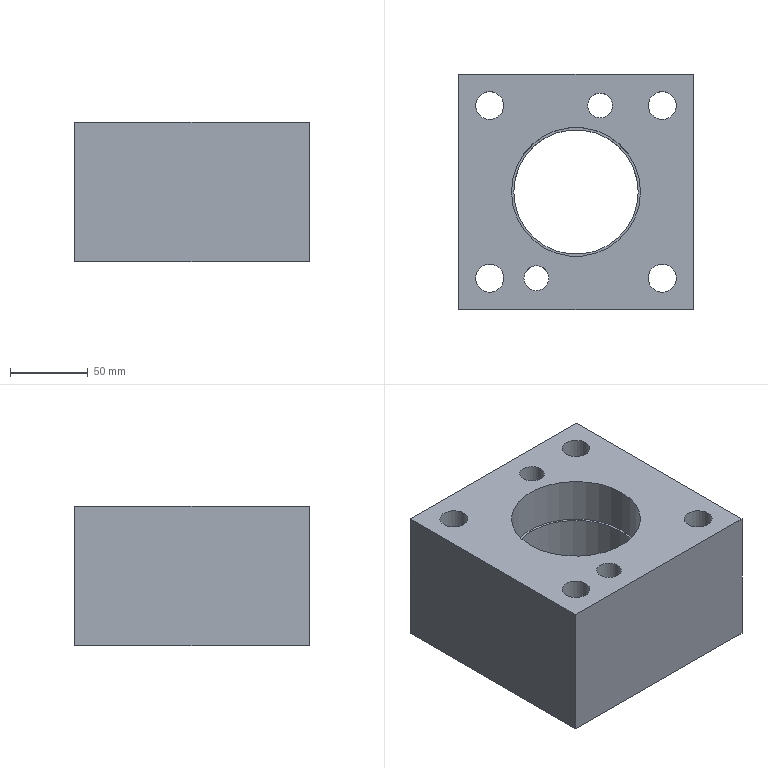Part | STEP file | lll_id766_x_t | 1 solid | 39 faces | box 151 x 151 x 90 mm | volume 1390274 mm3 | cylinder 20 | plane 13 | cone 6 | commonest cylinder face diameters 6.806 x4 18.009 x4 26.007 x4 10.505 x2 16 x2 18.5 x2
STEP:
#1=CARTESIAN_POINT('',(398.807,491.144,72.5));
#2=VERTEX_POINT('',#1);
#3=CARTESIAN_POINT('',(402.21,491.144,72.5));
#4=DIRECTION('',(0.,0.,-1.));
#5=DIRECTION('',(-1.,0.,0.));
#6=AXIS2_PLACEMENT_3D('',#3,#4,#5);
#7=CIRCLE('',#6,3.403);
#8=EDGE_CURVE('',#2,#2,#7,.T.);
#9=ORIENTED_EDGE('',*,*,#8,.F.);
#10=EDGE_LOOP('',(#9));
#11=FACE_BOUND('',#10,.T.);
#12=CARTESIAN_POINT('',(440.176,550.225,72.5));
#13=VERTEX_POINT('',#12);
#14=CARTESIAN_POINT('',(443.579,550.225,72.5));
#15=DIRECTION('',(0.,0.,-1.));
#16=DIRECTION('',(-1.,0.,0.));
#17=AXIS2_PLACEMENT_3D('',#14,#15,#16);
#18=CIRCLE('',#17,3.403);
#19=EDGE_CURVE('',#13,#13,#18,.T.);
#20=ORIENTED_EDGE('',*,*,#19,.F.);
#21=EDGE_LOOP('',(#20));
#22=FACE_BOUND('',#21,.T.);
#23=CARTESIAN_POINT('',(499.257,508.856,72.5));
#24=VERTEX_POINT('',#23);
#25=CARTESIAN_POINT('',(502.66,508.856,72.5));
#26=DIRECTION('',(0.,0.,-1.));
#27=DIRECTION('',(-1.,0.,0.));
#28=AXIS2_PLACEMENT_3D('',#25,#26,#27);
#29=CIRCLE('',#28,3.403);
#30=EDGE_CURVE('',#24,#24,#29,.T.);
#31=ORIENTED_EDGE('',*,*,#30,.F.);
#32=EDGE_LOOP('',(#31));
#33=FACE_BOUND('',#32,.T.);
#34=CARTESIAN_POINT('',(457.888,449.775,72.5));
#35=VERTEX_POINT('',#34);
#36=CARTESIAN_POINT('',(461.291,449.775,72.5));
#37=DIRECTION('',(0.,0.,-1.));
#38=DIRECTION('',(-1.,0.,0.));
#39=AXIS2_PLACEMENT_3D('',#36,#37,#38);
#40=CIRCLE('',#39,3.403);
#41=EDGE_CURVE('',#35,#35,#40,.T.);
#42=ORIENTED_EDGE('',*,*,#41,.F.);
#43=EDGE_LOOP('',(#42));
#44=FACE_BOUND('',#43,.T.);
#45=CARTESIAN_POINT('',(417.685,444.5,72.5));
#46=VERTEX_POINT('',#45);
#47=CARTESIAN_POINT('',(426.935,444.5,72.5));
#48=DIRECTION('',(0.,0.,-1.));
#49=DIRECTION('',(-1.,0.,0.));
#50=AXIS2_PLACEMENT_3D('',#47,#48,#49);
#51=CIRCLE('',#50,9.25);
#52=EDGE_CURVE('',#46,#46,#51,.T.);
#53=ORIENTED_EDGE('',*,*,#52,.F.);
#54=EDGE_LOOP('',(#53));
#55=FACE_BOUND('',#54,.T.);
#56=CARTESIAN_POINT('',(409.939,555.5,72.5));
#57=VERTEX_POINT('',#56);
#58=CARTESIAN_POINT('',(396.935,555.5,72.5));
#59=DIRECTION('',(0.,0.,1.));
#60=DIRECTION('',(1.,0.,0.));
#61=AXIS2_PLACEMENT_3D('',#58,#59,#60);
#62=CIRCLE('',#61,13.004);
#63=EDGE_CURVE('',#57,#57,#62,.T.);
#64=ORIENTED_EDGE('',*,*,#63,.T.);
#65=EDGE_LOOP('',(#64));
#66=FACE_BOUND('',#65,.T.);
#67=CARTESIAN_POINT('',(458.685,555.5,72.5));
#68=VERTEX_POINT('',#67);
#69=CARTESIAN_POINT('',(467.935,555.5,72.5));
#70=DIRECTION('',(0.,0.,-1.));
#71=DIRECTION('',(-1.,0.,0.));
#72=AXIS2_PLACEMENT_3D('',#69,#70,#71);
#73=CIRCLE('',#72,9.25);
#74=EDGE_CURVE('',#68,#68,#73,.T.);
#75=ORIENTED_EDGE('',*,*,#74,.F.);
#76=EDGE_LOOP('',(#75));
#77=FACE_BOUND('',#76,.T.);
#78=CARTESIAN_POINT('',(520.939,444.5,72.5));
#79=VERTEX_POINT('',#78);
#80=CARTESIAN_POINT('',(507.935,444.5,72.5));
#81=DIRECTION('',(0.,0.,1.));
#82=DIRECTION('',(1.,0.,0.));
#83=AXIS2_PLACEMENT_3D('',#80,#81,#82);
#84=CIRCLE('',#83,13.004);
#85=EDGE_CURVE('',#79,#79,#84,.T.);
#86=ORIENTED_EDGE('',*,*,#85,.T.);
#87=EDGE_LOOP('',(#86));
#88=FACE_BOUND('',#87,.T.);
#89=CARTESIAN_POINT('',(417.683,559.5,72.5));
#90=VERTEX_POINT('',#89);
#91=CARTESIAN_POINT('',(422.935,559.5,72.5));
#92=DIRECTION('',(0.,0.,-1.));
#93=DIRECTION('',(-1.,0.,0.));
#94=AXIS2_PLACEMENT_3D('',#91,#92,#93);
#95=CIRCLE('',#94,5.253);
#96=EDGE_CURVE('',#90,#90,#95,.T.);
#97=ORIENTED_EDGE('',*,*,#96,.F.);
#98=EDGE_LOOP('',(#97));
#99=FACE_BOUND('',#98,.T.);
#100=CARTESIAN_POINT('',(476.683,440.5,72.5));
#101=VERTEX_POINT('',#100);
#102=CARTESIAN_POINT('',(481.935,440.5,72.5));
#103=DIRECTION('',(0.,0.,-1.));
#104=DIRECTION('',(-1.,0.,0.));
#105=AXIS2_PLACEMENT_3D('',#102,#103,#104);
#106=CIRCLE('',#105,5.253);
#107=EDGE_CURVE('',#101,#101,#106,.T.);
#108=ORIENTED_EDGE('',*,*,#107,.F.);
#109=EDGE_LOOP('',(#108));
#110=FACE_BOUND('',#109,.T.);
#111=CARTESIAN_POINT('',(376.935,424.5,72.5));
#112=VERTEX_POINT('',#111);
#113=CARTESIAN_POINT('',(527.935,424.5,72.5));
#114=VERTEX_POINT('',#113);
#115=CARTESIAN_POINT('',(452.435,424.5,72.5));
#116=DIRECTION('',(1.,0.,0.));
#117=VECTOR('',#116,1.);
#118=LINE('',#115,#117);
#119=EDGE_CURVE('',#112,#114,#118,.T.);
#120=ORIENTED_EDGE('',*,*,#119,.F.);
#121=CARTESIAN_POINT('',(376.935,575.5,72.5));
#122=VERTEX_POINT('',#121);
#123=CARTESIAN_POINT('',(376.935,0.,72.5));
#124=DIRECTION('',(0.,1.,0.));
#125=VECTOR('',#124,1.);
#126=LINE('',#123,#125);
#127=EDGE_CURVE('',#112,#122,#126,.T.);
#128=ORIENTED_EDGE('',*,*,#127,.T.);
#129=CARTESIAN_POINT('',(527.935,575.5,72.5));
#130=VERTEX_POINT('',#129);
#131=CARTESIAN_POINT('',(452.435,575.5,72.5));
#132=DIRECTION('',(-1.,0.,0.));
#133=VECTOR('',#132,1.);
#134=LINE('',#131,#133);
#135=EDGE_CURVE('',#130,#122,#134,.T.);
#136=ORIENTED_EDGE('',*,*,#135,.F.);
#137=CARTESIAN_POINT('',(527.935,0.,72.5));
#138=DIRECTION('',(0.,-1.,0.));
#139=VECTOR('',#138,1.);
#140=LINE('',#137,#139);
#141=EDGE_CURVE('',#130,#114,#140,.T.);
#142=ORIENTED_EDGE('',*,*,#141,.T.);
#143=EDGE_LOOP('',(#120,#128,#136,#142));
#144=FACE_BOUND('',#143,.T.);
#145=CARTESIAN_POINT('',(492.435,500.,72.5));
#146=VERTEX_POINT('',#145);
#147=CARTESIAN_POINT('',(452.435,500.,72.5));
#148=DIRECTION('',(0.,0.,1.));
#149=DIRECTION('',(1.,0.,0.));
#150=AXIS2_PLACEMENT_3D('',#147,#148,#149);
#151=CIRCLE('',#150,40.);
#152=EDGE_CURVE('',#146,#146,#151,.T.);
#153=ORIENTED_EDGE('',*,*,#152,.T.);
#154=EDGE_LOOP('',(#153));
#155=FACE_BOUND('',#154,.T.);
#156=CARTESIAN_POINT('',(520.939,555.5,72.5));
#157=VERTEX_POINT('',#156);
#158=CARTESIAN_POINT('',(507.935,555.5,72.5));
#159=DIRECTION('',(0.,0.,1.));
#160=DIRECTION('',(1.,0.,0.));
#161=AXIS2_PLACEMENT_3D('',#158,#159,#160);
#162=CIRCLE('',#161,13.004);
#163=EDGE_CURVE('',#157,#157,#162,.T.);
#164=ORIENTED_EDGE('',*,*,#163,.T.);
#165=EDGE_LOOP('',(#164));
#166=FACE_BOUND('',#165,.T.);
#167=CARTESIAN_POINT('',(409.939,444.5,72.5));
#168=VERTEX_POINT('',#167);
#169=CARTESIAN_POINT('',(396.935,444.5,72.5));
#170=DIRECTION('',(0.,0.,1.));
#171=DIRECTION('',(1.,0.,0.));
#172=AXIS2_PLACEMENT_3D('',#169,#170,#171);
#173=CIRCLE('',#172,13.004);
#174=EDGE_CURVE('',#168,#168,#173,.T.);
#175=ORIENTED_EDGE('',*,*,#174,.T.);
#176=EDGE_LOOP('',(#175));
#177=FACE_BOUND('',#176,.T.);
#178=CARTESIAN_POINT('',(2067.435,0.,72.5));
#179=DIRECTION('',(0.,0.,-1.));
#180=DIRECTION('',(-1.,0.,0.));
#181=AXIS2_PLACEMENT_3D('',#178,#179,#180);
#182=PLANE('',#181);
#183=ADVANCED_FACE('',(#11,#22,#33,#44,#55,#66,#77,#88,#99,#110,#144,#155,#166,#177),#182,.T.);
#184=CARTESIAN_POINT('',(418.935,444.5,162.5));
#185=VERTEX_POINT('',#184);
#186=CARTESIAN_POINT('',(426.935,444.5,162.5));
#187=DIRECTION('',(0.,0.,-1.));
#188=DIRECTION('',(-1.,0.,0.));
#189=AXIS2_PLACEMENT_3D('',#186,#187,#188);
#190=CIRCLE('',#189,8.);
#191=EDGE_CURVE('',#185,#185,#190,.T.);
#192=ORIENTED_EDGE('',*,*,#191,.T.);
#193=EDGE_LOOP('',(#192));
#194=FACE_BOUND('',#193,.T.);
#195=CARTESIAN_POINT('',(387.931,444.5,162.5));
#196=VERTEX_POINT('',#195);
#197=CARTESIAN_POINT('',(396.935,444.5,162.5));
#198=DIRECTION('',(0.,0.,-1.));
#199=DIRECTION('',(-1.,0.,0.));
#200=AXIS2_PLACEMENT_3D('',#197,#198,#199);
#201=CIRCLE('',#200,9.005);
#202=EDGE_CURVE('',#196,#196,#201,.T.);
#203=ORIENTED_EDGE('',*,*,#202,.T.);
#204=EDGE_LOOP('',(#203));
#205=FACE_BOUND('',#204,.T.);
#206=CARTESIAN_POINT('',(387.931,555.5,162.5));
#207=VERTEX_POINT('',#206);
#208=CARTESIAN_POINT('',(396.935,555.5,162.5));
#209=DIRECTION('',(0.,0.,-1.));
#210=DIRECTION('',(-1.,0.,0.));
#211=AXIS2_PLACEMENT_3D('',#208,#209,#210);
#212=CIRCLE('',#211,9.005);
#213=EDGE_CURVE('',#207,#207,#212,.T.);
#214=ORIENTED_EDGE('',*,*,#213,.T.);
#215=EDGE_LOOP('',(#214));
#216=FACE_BOUND('',#215,.T.);
#217=CARTESIAN_POINT('',(459.935,555.5,162.5));
#218=VERTEX_POINT('',#217);
#219=CARTESIAN_POINT('',(467.935,555.5,162.5));
#220=DIRECTION('',(0.,0.,-1.));
#221=DIRECTION('',(-1.,0.,0.));
#222=AXIS2_PLACEMENT_3D('',#219,#220,#221);
#223=CIRCLE('',#222,8.);
#224=EDGE_CURVE('',#218,#218,#223,.T.);
#225=ORIENTED_EDGE('',*,*,#224,.T.);
#226=EDGE_LOOP('',(#225));
#227=FACE_BOUND('',#226,.T.);
#228=CARTESIAN_POINT('',(498.931,555.5,162.5));
#229=VERTEX_POINT('',#228);
#230=CARTESIAN_POINT('',(507.935,555.5,162.5));
#231=DIRECTION('',(0.,0.,-1.));
#232=DIRECTION('',(-1.,0.,0.));
#233=AXIS2_PLACEMENT_3D('',#230,#231,#232);
#234=CIRCLE('',#233,9.005);
#235=EDGE_CURVE('',#229,#229,#234,.T.);
#236=ORIENTED_EDGE('',*,*,#235,.T.);
#237=EDGE_LOOP('',(#236));
#238=FACE_BOUND('',#237,.T.);
#239=CARTESIAN_POINT('',(498.931,444.5,162.5));
#240=VERTEX_POINT('',#239);
#241=CARTESIAN_POINT('',(507.935,444.5,162.5));
#242=DIRECTION('',(0.,0.,-1.));
#243=DIRECTION('',(-1.,0.,0.));
#244=AXIS2_PLACEMENT_3D('',#241,#242,#243);
#245=CIRCLE('',#244,9.005);
#246=EDGE_CURVE('',#240,#240,#245,.T.);
#247=ORIENTED_EDGE('',*,*,#246,.T.);
#248=EDGE_LOOP('',(#247));
#249=FACE_BOUND('',#248,.T.);
#250=CARTESIAN_POINT('',(410.935,500.,162.5));
#251=VERTEX_POINT('',#250);
#252=CARTESIAN_POINT('',(452.435,500.,162.5));
#253=DIRECTION('',(0.,0.,-1.));
#254=DIRECTION('',(-1.,0.,0.));
#255=AXIS2_PLACEMENT_3D('',#252,#253,#254);
#256=CIRCLE('',#255,41.5);
#257=EDGE_CURVE('',#251,#251,#256,.T.);
#258=ORIENTED_EDGE('',*,*,#257,.T.);
#259=EDGE_LOOP('',(#258));
#260=FACE_BOUND('',#259,.T.);
#261=CARTESIAN_POINT('',(527.935,424.5,162.5));
#262=VERTEX_POINT('',#261);
#263=CARTESIAN_POINT('',(376.935,424.5,162.5));
#264=VERTEX_POINT('',#263);
#265=CARTESIAN_POINT('',(2067.435,424.5,162.5));
#266=DIRECTION('',(-1.,0.,0.));
#267=VECTOR('',#266,1.);
#268=LINE('',#265,#267);
#269=EDGE_CURVE('',#262,#264,#268,.T.);
#270=ORIENTED_EDGE('',*,*,#269,.F.);
#271=CARTESIAN_POINT('',(527.935,575.5,162.5));
#272=VERTEX_POINT('',#271);
#273=CARTESIAN_POINT('',(527.935,500.,162.5));
#274=DIRECTION('',(0.,1.,0.));
#275=VECTOR('',#274,1.);
#276=LINE('',#273,#275);
#277=EDGE_CURVE('',#262,#272,#276,.T.);
#278=ORIENTED_EDGE('',*,*,#277,.T.);
#279=CARTESIAN_POINT('',(376.935,575.5,162.5));
#280=VERTEX_POINT('',#279);
#281=CARTESIAN_POINT('',(452.435,575.5,162.5));
#282=DIRECTION('',(-1.,0.,0.));
#283=VECTOR('',#282,1.);
#284=LINE('',#281,#283);
#285=EDGE_CURVE('',#272,#280,#284,.T.);
#286=ORIENTED_EDGE('',*,*,#285,.T.);
#287=CARTESIAN_POINT('',(376.935,500.,162.5));
#288=DIRECTION('',(0.,-1.,0.));
#289=VECTOR('',#288,1.);
#290=LINE('',#287,#289);
#291=EDGE_CURVE('',#280,#264,#290,.T.);
#292=ORIENTED_EDGE('',*,*,#291,.T.);
#293=EDGE_LOOP('',(#270,#278,#286,#292));
#294=FACE_BOUND('',#293,.T.);
#295=CARTESIAN_POINT('',(2067.435,0.,162.5));
#296=DIRECTION('',(0.,0.,-1.));
#297=DIRECTION('',(-1.,0.,0.));
#298=AXIS2_PLACEMENT_3D('',#295,#296,#297);
#299=PLANE('',#298);
#300=ADVANCED_FACE('',(#194,#205,#216,#227,#238,#249,#260,#294),#299,.F.);
#301=CARTESIAN_POINT('',(527.935,424.5,89.));
#302=DIRECTION('',(0.,0.,1.));
#303=VECTOR('',#302,1.);
#304=LINE('',#301,#303);
#305=EDGE_CURVE('',#114,#262,#304,.T.);
#306=ORIENTED_EDGE('',*,*,#305,.F.);
#307=ORIENTED_EDGE('',*,*,#141,.F.);
#308=CARTESIAN_POINT('',(527.935,575.5,89.));
#309=DIRECTION('',(0.,0.,1.));
#310=VECTOR('',#309,1.);
#311=LINE('',#308,#310);
#312=EDGE_CURVE('',#130,#272,#311,.T.);
#313=ORIENTED_EDGE('',*,*,#312,.T.);
#314=ORIENTED_EDGE('',*,*,#277,.F.);
#315=EDGE_LOOP('',(#306,#307,#313,#314));
#316=FACE_OUTER_BOUND('',#315,.T.);
#317=CARTESIAN_POINT('',(527.935,500.,89.));
#318=DIRECTION('',(1.,0.,0.));
#319=DIRECTION('',(0.,0.,-1.));
#320=AXIS2_PLACEMENT_3D('',#317,#318,#319);
#321=PLANE('',#320);
#322=ADVANCED_FACE('',(#316),#321,.T.);
#323=ORIENTED_EDGE('',*,*,#312,.F.);
#324=ORIENTED_EDGE('',*,*,#135,.T.);
#325=CARTESIAN_POINT('',(376.935,575.5,89.));
#326=DIRECTION('',(0.,0.,1.));
#327=VECTOR('',#326,1.);
#328=LINE('',#325,#327);
#329=EDGE_CURVE('',#122,#280,#328,.T.);
#330=ORIENTED_EDGE('',*,*,#329,.T.);
#331=ORIENTED_EDGE('',*,*,#285,.F.);
#332=EDGE_LOOP('',(#323,#324,#330,#331));
#333=FACE_OUTER_BOUND('',#332,.T.);
#334=CARTESIAN_POINT('',(452.435,575.5,89.));
#335=DIRECTION('',(0.,1.,0.));
#336=DIRECTION('',(0.,0.,1.));
#337=AXIS2_PLACEMENT_3D('',#334,#335,#336);
#338=PLANE('',#337);
#339=ADVANCED_FACE('',(#333),#338,.T.);
#340=ORIENTED_EDGE('',*,*,#329,.F.);
#341=ORIENTED_EDGE('',*,*,#127,.F.);
#342=CARTESIAN_POINT('',(376.935,424.5,89.));
#343=DIRECTION('',(0.,0.,1.));
#344=VECTOR('',#343,1.);
#345=LINE('',#342,#344);
#346=EDGE_CURVE('',#112,#264,#345,.T.);
#347=ORIENTED_EDGE('',*,*,#346,.T.);
#348=ORIENTED_EDGE('',*,*,#291,.F.);
#349=EDGE_LOOP('',(#340,#341,#347,#348));
#350=FACE_OUTER_BOUND('',#349,.T.);
#351=CARTESIAN_POINT('',(376.935,500.,89.));
#352=DIRECTION('',(-1.,0.,0.));
#353=DIRECTION('',(0.,0.,1.));
#354=AXIS2_PLACEMENT_3D('',#351,#352,#353);
#355=PLANE('',#354);
#356=ADVANCED_FACE('',(#350),#355,.T.);
#357=ORIENTED_EDGE('',*,*,#346,.F.);
#358=ORIENTED_EDGE('',*,*,#119,.T.);
#359=ORIENTED_EDGE('',*,*,#305,.T.);
#360=ORIENTED_EDGE('',*,*,#269,.T.);
#361=EDGE_LOOP('',(#357,#358,#359,#360));
#362=FACE_OUTER_BOUND('',#361,.T.);
#363=CARTESIAN_POINT('',(452.435,424.5,89.));
#364=DIRECTION('',(0.,-1.,0.));
#365=DIRECTION('',(0.,0.,-1.));
#366=AXIS2_PLACEMENT_3D('',#363,#364,#365);
#367=PLANE('',#366);
#368=ADVANCED_FACE('',(#362),#367,.T.);
#369=CARTESIAN_POINT('',(492.435,500.,133.));
#370=VERTEX_POINT('',#369);
#371=CARTESIAN_POINT('',(452.435,500.,133.));
#372=DIRECTION('',(0.,0.,-1.));
#373=DIRECTION('',(1.,0.,0.));
#374=AXIS2_PLACEMENT_3D('',#371,#372,#373);
#375=CIRCLE('',#374,40.);
#376=EDGE_CURVE('',#370,#370,#375,.T.);
#377=ORIENTED_EDGE('',*,*,#376,.F.);
#378=EDGE_LOOP('',(#377));
#379=FACE_BOUND('',#378,.T.);
#380=ORIENTED_EDGE('',*,*,#152,.F.);
#381=EDGE_LOOP('',(#380));
#382=FACE_BOUND('',#381,.T.);
#383=CARTESIAN_POINT('',(452.435,500.,317.5));
#384=DIRECTION('',(0.,0.,-1.));
#385=DIRECTION('',(-1.,0.,0.));
#386=AXIS2_PLACEMENT_3D('',#383,#384,#385);
#387=CYLINDRICAL_SURFACE('',#386,40.);
#388=ADVANCED_FACE('',(#379,#382),#387,.F.);
#389=CARTESIAN_POINT('',(493.935,500.,133.));
#390=VERTEX_POINT('',#389);
#391=CARTESIAN_POINT('',(452.435,500.,133.));
#392=DIRECTION('',(0.,0.,-1.));
#393=DIRECTION('',(1.,0.,0.));
#394=AXIS2_PLACEMENT_3D('',#391,#392,#393);
#395=CIRCLE('',#394,41.5);
#396=EDGE_CURVE('',#390,#390,#395,.T.);
#397=ORIENTED_EDGE('',*,*,#396,.T.);
#398=EDGE_LOOP('',(#397));
#399=FACE_BOUND('',#398,.T.);
#400=ORIENTED_EDGE('',*,*,#257,.F.);
#401=EDGE_LOOP('',(#400));
#402=FACE_BOUND('',#401,.T.);
#403=CARTESIAN_POINT('',(452.435,500.,153.));
#404=DIRECTION('',(0.,0.,-1.));
#405=DIRECTION('',(-1.,0.,0.));
#406=AXIS2_PLACEMENT_3D('',#403,#404,#405);
#407=CYLINDRICAL_SURFACE('',#406,41.5);
#408=ADVANCED_FACE('',(#399,#402),#407,.F.);
#409=ORIENTED_EDGE('',*,*,#376,.T.);
#410=EDGE_LOOP('',(#409));
#411=FACE_BOUND('',#410,.T.);
#412=ORIENTED_EDGE('',*,*,#396,.F.);
#413=EDGE_LOOP('',(#412));
#414=FACE_BOUND('',#413,.T.);
#415=CARTESIAN_POINT('',(452.435,500.,133.));
#416=DIRECTION('',(0.,0.,1.));
#417=DIRECTION('',(-1.,0.,0.));
#418=AXIS2_PLACEMENT_3D('',#415,#416,#417);
#419=PLANE('',#418);
#420=ADVANCED_FACE('',(#411,#414),#419,.T.);
#421=ORIENTED_EDGE('',*,*,#107,.T.);
#422=EDGE_LOOP('',(#421));
#423=FACE_BOUND('',#422,.T.);
#424=CARTESIAN_POINT('',(487.188,440.5,102.253));
#425=VERTEX_POINT('',#424);
#426=CARTESIAN_POINT('',(481.935,440.5,102.253));
#427=DIRECTION('',(0.,0.,1.));
#428=DIRECTION('',(1.,0.,0.));
#429=AXIS2_PLACEMENT_3D('',#426,#427,#428);
#430=CIRCLE('',#429,5.253);
#431=EDGE_CURVE('',#425,#425,#430,.T.);
#432=ORIENTED_EDGE('',*,*,#431,.T.);
#433=EDGE_LOOP('',(#432));
#434=FACE_BOUND('',#433,.T.);
#435=CARTESIAN_POINT('',(481.935,440.5,67.5));
#436=DIRECTION('',(0.,0.,1.));
#437=DIRECTION('',(1.,0.,0.));
#438=AXIS2_PLACEMENT_3D('',#435,#436,#437);
#439=CYLINDRICAL_SURFACE('',#438,5.253);
#440=ADVANCED_FACE('',(#423,#434),#439,.F.);
#441=CARTESIAN_POINT('',(481.935,440.5,107.506));
#442=VERTEX_POINT('',#441);
#443=VERTEX_LOOP('',#442);
#444=FACE_BOUND('',#443,.T.);
#445=ORIENTED_EDGE('',*,*,#431,.F.);
#446=EDGE_LOOP('',(#445));
#447=FACE_BOUND('',#446,.T.);
#448=CARTESIAN_POINT('',(481.935,440.5,102.253));
#449=DIRECTION('',(0.,0.,-1.));
#450=DIRECTION('',(-1.,0.,0.));
#451=AXIS2_PLACEMENT_3D('',#448,#449,#450);
#452=CONICAL_SURFACE('',#451,5.253,45.);
#453=ADVANCED_FACE('',(#444,#447),#452,.F.);
#454=ORIENTED_EDGE('',*,*,#96,.T.);
#455=EDGE_LOOP('',(#454));
#456=FACE_BOUND('',#455,.T.);
#457=CARTESIAN_POINT('',(428.188,559.5,102.253));
#458=VERTEX_POINT('',#457);
#459=CARTESIAN_POINT('',(422.935,559.5,102.253));
#460=DIRECTION('',(0.,0.,1.));
#461=DIRECTION('',(1.,0.,0.));
#462=AXIS2_PLACEMENT_3D('',#459,#460,#461);
#463=CIRCLE('',#462,5.253);
#464=EDGE_CURVE('',#458,#458,#463,.T.);
#465=ORIENTED_EDGE('',*,*,#464,.T.);
#466=EDGE_LOOP('',(#465));
#467=FACE_BOUND('',#466,.T.);
#468=CARTESIAN_POINT('',(422.935,559.5,67.5));
#469=DIRECTION('',(0.,0.,1.));
#470=DIRECTION('',(1.,0.,0.));
#471=AXIS2_PLACEMENT_3D('',#468,#469,#470);
#472=CYLINDRICAL_SURFACE('',#471,5.253);
#473=ADVANCED_FACE('',(#456,#467),#472,.F.);
#474=CARTESIAN_POINT('',(422.935,559.5,107.506));
#475=VERTEX_POINT('',#474);
#476=VERTEX_LOOP('',#475);
#477=FACE_BOUND('',#476,.T.);
#478=ORIENTED_EDGE('',*,*,#464,.F.);
#479=EDGE_LOOP('',(#478));
#480=FACE_BOUND('',#479,.T.);
#481=CARTESIAN_POINT('',(422.935,559.5,102.253));
#482=DIRECTION('',(0.,0.,-1.));
#483=DIRECTION('',(-1.,0.,0.));
#484=AXIS2_PLACEMENT_3D('',#481,#482,#483);
#485=CONICAL_SURFACE('',#484,5.253,45.);
#486=ADVANCED_FACE('',(#477,#480),#485,.F.);
#487=CARTESIAN_POINT('',(516.94,444.5,122.5));
#488=VERTEX_POINT('',#487);
#489=CARTESIAN_POINT('',(507.935,444.5,122.5));
#490=DIRECTION('',(0.,0.,1.));
#491=DIRECTION('',(1.,0.,0.));
#492=AXIS2_PLACEMENT_3D('',#489,#490,#491);
#493=CIRCLE('',#492,9.005);
#494=EDGE_CURVE('',#488,#488,#493,.T.);
#495=ORIENTED_EDGE('',*,*,#494,.F.);
#496=EDGE_LOOP('',(#495));
#497=FACE_BOUND('',#496,.T.);
#498=ORIENTED_EDGE('',*,*,#246,.F.);
#499=EDGE_LOOP('',(#498));
#500=FACE_BOUND('',#499,.T.);
#501=CARTESIAN_POINT('',(507.935,444.5,67.5));
#502=DIRECTION('',(0.,0.,1.));
#503=DIRECTION('',(-1.,0.,0.));
#504=AXIS2_PLACEMENT_3D('',#501,#502,#503);
#505=CYLINDRICAL_SURFACE('',#504,9.005);
#506=ADVANCED_FACE('',(#497,#500),#505,.F.);
#507=ORIENTED_EDGE('',*,*,#494,.T.);
#508=EDGE_LOOP('',(#507));
#509=FACE_BOUND('',#508,.T.);
#510=CARTESIAN_POINT('',(520.939,444.5,122.5));
#511=VERTEX_POINT('',#510);
#512=CARTESIAN_POINT('',(507.935,444.5,122.5));
#513=DIRECTION('',(0.,0.,1.));
#514=DIRECTION('',(1.,0.,0.));
#515=AXIS2_PLACEMENT_3D('',#512,#513,#514);
#516=CIRCLE('',#515,13.004);
#517=EDGE_CURVE('',#511,#511,#516,.T.);
#518=ORIENTED_EDGE('',*,*,#517,.F.);
#519=EDGE_LOOP('',(#518));
#520=FACE_BOUND('',#519,.T.);
#521=CARTESIAN_POINT('',(507.935,444.5,122.5));
#522=DIRECTION('',(0.,0.,1.));
#523=DIRECTION('',(-1.,0.,0.));
#524=AXIS2_PLACEMENT_3D('',#521,#522,#523);
#525=PLANE('',#524);
#526=ADVANCED_FACE('',(#509,#520),#525,.F.);
#527=ORIENTED_EDGE('',*,*,#517,.T.);
#528=EDGE_LOOP('',(#527));
#529=FACE_BOUND('',#528,.T.);
#530=ORIENTED_EDGE('',*,*,#85,.F.);
#531=EDGE_LOOP('',(#530));
#532=FACE_BOUND('',#531,.T.);
#533=CARTESIAN_POINT('',(507.935,444.5,72.5));
#534=DIRECTION('',(0.,0.,1.));
#535=DIRECTION('',(-1.,0.,0.));
#536=AXIS2_PLACEMENT_3D('',#533,#534,#535);
#537=CYLINDRICAL_SURFACE('',#536,13.004);
#538=ADVANCED_FACE('',(#529,#532),#537,.F.);
#539=CARTESIAN_POINT('',(516.94,555.5,122.5));
#540=VERTEX_POINT('',#539);
#541=CARTESIAN_POINT('',(507.935,555.5,122.5));
#542=DIRECTION('',(0.,0.,1.));
#543=DIRECTION('',(1.,0.,0.));
#544=AXIS2_PLACEMENT_3D('',#541,#542,#543);
#545=CIRCLE('',#544,9.005);
#546=EDGE_CURVE('',#540,#540,#545,.T.);
#547=ORIENTED_EDGE('',*,*,#546,.F.);
#548=EDGE_LOOP('',(#547));
#549=FACE_BOUND('',#548,.T.);
#550=ORIENTED_EDGE('',*,*,#235,.F.);
#551=EDGE_LOOP('',(#550));
#552=FACE_BOUND('',#551,.T.);
#553=CARTESIAN_POINT('',(507.935,555.5,67.5));
#554=DIRECTION('',(0.,0.,1.));
#555=DIRECTION('',(-1.,0.,0.));
#556=AXIS2_PLACEMENT_3D('',#553,#554,#555);
#557=CYLINDRICAL_SURFACE('',#556,9.005);
#558=ADVANCED_FACE('',(#549,#552),#557,.F.);
#559=ORIENTED_EDGE('',*,*,#546,.T.);
#560=EDGE_LOOP('',(#559));
#561=FACE_BOUND('',#560,.T.);
#562=CARTESIAN_POINT('',(520.939,555.5,122.5));
#563=VERTEX_POINT('',#562);
#564=CARTESIAN_POINT('',(507.935,555.5,122.5));
#565=DIRECTION('',(0.,0.,1.));
#566=DIRECTION('',(1.,0.,0.));
#567=AXIS2_PLACEMENT_3D('',#564,#565,#566);
#568=CIRCLE('',#567,13.004);
#569=EDGE_CURVE('',#563,#563,#568,.T.);
#570=ORIENTED_EDGE('',*,*,#569,.F.);
#571=EDGE_LOOP('',(#570));
#572=FACE_BOUND('',#571,.T.);
#573=CARTESIAN_POINT('',(507.935,555.5,122.5));
#574=DIRECTION('',(0.,0.,1.));
#575=DIRECTION('',(-1.,0.,0.));
#576=AXIS2_PLACEMENT_3D('',#573,#574,#575);
#577=PLANE('',#576);
#578=ADVANCED_FACE('',(#561,#572),#577,.F.);
#579=ORIENTED_EDGE('',*,*,#569,.T.);
#580=EDGE_LOOP('',(#579));
#581=FACE_BOUND('',#580,.T.);
#582=ORIENTED_EDGE('',*,*,#163,.F.);
#583=EDGE_LOOP('',(#582));
#584=FACE_BOUND('',#583,.T.);
#585=CARTESIAN_POINT('',(507.935,555.5,72.5));
#586=DIRECTION('',(0.,0.,1.));
#587=DIRECTION('',(-1.,0.,0.));
#588=AXIS2_PLACEMENT_3D('',#585,#586,#587);
#589=CYLINDRICAL_SURFACE('',#588,13.004);
#590=ADVANCED_FACE('',(#581,#584),#589,.F.);
#591=CARTESIAN_POINT('',(475.935,555.5,113.5));
#592=VERTEX_POINT('',#591);
#593=CARTESIAN_POINT('',(467.935,555.5,113.5));
#594=DIRECTION('',(0.,0.,1.));
#595=DIRECTION('',(1.,0.,0.));
#596=AXIS2_PLACEMENT_3D('',#593,#594,#595);
#597=CIRCLE('',#596,8.);
#598=EDGE_CURVE('',#592,#592,#597,.T.);
#599=ORIENTED_EDGE('',*,*,#598,.F.);
#600=EDGE_LOOP('',(#599));
#601=FACE_BOUND('',#600,.T.);
#602=ORIENTED_EDGE('',*,*,#224,.F.);
#603=EDGE_LOOP('',(#602));
#604=FACE_BOUND('',#603,.T.);
#605=CARTESIAN_POINT('',(467.935,555.5,67.5));
#606=DIRECTION('',(0.,0.,1.));
#607=DIRECTION('',(-1.,0.,0.));
#608=AXIS2_PLACEMENT_3D('',#605,#606,#607);
#609=CYLINDRICAL_SURFACE('',#608,8.);
#610=ADVANCED_FACE('',(#601,#604),#609,.F.);
#611=ORIENTED_EDGE('',*,*,#598,.T.);
#612=EDGE_LOOP('',(#611));
#613=FACE_BOUND('',#612,.T.);
#614=CARTESIAN_POINT('',(477.185,555.5,113.5));
#615=VERTEX_POINT('',#614);
#616=CARTESIAN_POINT('',(467.935,555.5,113.5));
#617=DIRECTION('',(0.,0.,1.));
#618=DIRECTION('',(1.,0.,0.));
#619=AXIS2_PLACEMENT_3D('',#616,#617,#618);
#620=CIRCLE('',#619,9.25);
#621=EDGE_CURVE('',#615,#615,#620,.T.);
#622=ORIENTED_EDGE('',*,*,#621,.F.);
#623=EDGE_LOOP('',(#622));
#624=FACE_BOUND('',#623,.T.);
#625=CARTESIAN_POINT('',(467.935,555.5,113.5));
#626=DIRECTION('',(0.,0.,1.));
#627=DIRECTION('',(-1.,0.,0.));
#628=AXIS2_PLACEMENT_3D('',#625,#626,#627);
#629=PLANE('',#628);
#630=ADVANCED_FACE('',(#613,#624),#629,.F.);
#631=ORIENTED_EDGE('',*,*,#74,.T.);
#632=EDGE_LOOP('',(#631));
#633=FACE_BOUND('',#632,.T.);
#634=ORIENTED_EDGE('',*,*,#621,.T.);
#635=EDGE_LOOP('',(#634));
#636=FACE_BOUND('',#635,.T.);
#637=CARTESIAN_POINT('',(467.935,555.5,67.5));
#638=DIRECTION('',(0.,0.,1.));
#639=DIRECTION('',(-1.,0.,0.));
#640=AXIS2_PLACEMENT_3D('',#637,#638,#639);
#641=CYLINDRICAL_SURFACE('',#640,9.25);
#642=ADVANCED_FACE('',(#633,#636),#641,.F.);
#643=CARTESIAN_POINT('',(405.94,555.5,122.5));
#644=VERTEX_POINT('',#643);
#645=CARTESIAN_POINT('',(396.935,555.5,122.5));
#646=DIRECTION('',(0.,0.,1.));
#647=DIRECTION('',(1.,0.,0.));
#648=AXIS2_PLACEMENT_3D('',#645,#646,#647);
#649=CIRCLE('',#648,9.005);
#650=EDGE_CURVE('',#644,#644,#649,.T.);
#651=ORIENTED_EDGE('',*,*,#650,.F.);
#652=EDGE_LOOP('',(#651));
#653=FACE_BOUND('',#652,.T.);
#654=ORIENTED_EDGE('',*,*,#213,.F.);
#655=EDGE_LOOP('',(#654));
#656=FACE_BOUND('',#655,.T.);
#657=CARTESIAN_POINT('',(396.935,555.5,67.5));
#658=DIRECTION('',(0.,0.,1.));
#659=DIRECTION('',(-1.,0.,0.));
#660=AXIS2_PLACEMENT_3D('',#657,#658,#659);
#661=CYLINDRICAL_SURFACE('',#660,9.005);
#662=ADVANCED_FACE('',(#653,#656),#661,.F.);
#663=ORIENTED_EDGE('',*,*,#650,.T.);
#664=EDGE_LOOP('',(#663));
#665=FACE_BOUND('',#664,.T.);
#666=CARTESIAN_POINT('',(409.939,555.5,122.5));
#667=VERTEX_POINT('',#666);
#668=CARTESIAN_POINT('',(396.935,555.5,122.5));
#669=DIRECTION('',(0.,0.,1.));
#670=DIRECTION('',(1.,0.,0.));
#671=AXIS2_PLACEMENT_3D('',#668,#669,#670);
#672=CIRCLE('',#671,13.004);
#673=EDGE_CURVE('',#667,#667,#672,.T.);
#674=ORIENTED_EDGE('',*,*,#673,.F.);
#675=EDGE_LOOP('',(#674));
#676=FACE_BOUND('',#675,.T.);
#677=CARTESIAN_POINT('',(396.935,555.5,122.5));
#678=DIRECTION('',(0.,0.,1.));
#679=DIRECTION('',(-1.,0.,0.));
#680=AXIS2_PLACEMENT_3D('',#677,#678,#679);
#681=PLANE('',#680);
#682=ADVANCED_FACE('',(#665,#676),#681,.F.);
#683=ORIENTED_EDGE('',*,*,#673,.T.);
#684=EDGE_LOOP('',(#683));
#685=FACE_BOUND('',#684,.T.);
#686=ORIENTED_EDGE('',*,*,#63,.F.);
#687=EDGE_LOOP('',(#686));
#688=FACE_BOUND('',#687,.T.);
#689=CARTESIAN_POINT('',(396.935,555.5,72.5));
#690=DIRECTION('',(0.,0.,1.));
#691=DIRECTION('',(-1.,0.,0.));
#692=AXIS2_PLACEMENT_3D('',#689,#690,#691);
#693=CYLINDRICAL_SURFACE('',#692,13.004);
#694=ADVANCED_FACE('',(#685,#688),#693,.F.);
#695=CARTESIAN_POINT('',(405.94,444.5,122.5));
#696=VERTEX_POINT('',#695);
#697=CARTESIAN_POINT('',(396.935,444.5,122.5));
#698=DIRECTION('',(0.,0.,1.));
#699=DIRECTION('',(1.,0.,0.));
#700=AXIS2_PLACEMENT_3D('',#697,#698,#699);
#701=CIRCLE('',#700,9.005);
#702=EDGE_CURVE('',#696,#696,#701,.T.);
#703=ORIENTED_EDGE('',*,*,#702,.F.);
#704=EDGE_LOOP('',(#703));
#705=FACE_BOUND('',#704,.T.);
#706=ORIENTED_EDGE('',*,*,#202,.F.);
#707=EDGE_LOOP('',(#706));
#708=FACE_BOUND('',#707,.T.);
#709=CARTESIAN_POINT('',(396.935,444.5,67.5));
#710=DIRECTION('',(0.,0.,1.));
#711=DIRECTION('',(-1.,0.,0.));
#712=AXIS2_PLACEMENT_3D('',#709,#710,#711);
#713=CYLINDRICAL_SURFACE('',#712,9.005);
#714=ADVANCED_FACE('',(#705,#708),#713,.F.);
#715=ORIENTED_EDGE('',*,*,#702,.T.);
#716=EDGE_LOOP('',(#715));
#717=FACE_BOUND('',#716,.T.);
#718=CARTESIAN_POINT('',(409.939,444.5,122.5));
#719=VERTEX_POINT('',#718);
#720=CARTESIAN_POINT('',(396.935,444.5,122.5));
#721=DIRECTION('',(0.,0.,1.));
#722=DIRECTION('',(1.,0.,0.));
#723=AXIS2_PLACEMENT_3D('',#720,#721,#722);
#724=CIRCLE('',#723,13.004);
#725=EDGE_CURVE('',#719,#719,#724,.T.);
#726=ORIENTED_EDGE('',*,*,#725,.F.);
#727=EDGE_LOOP('',(#726));
#728=FACE_BOUND('',#727,.T.);
#729=CARTESIAN_POINT('',(396.935,444.5,122.5));
#730=DIRECTION('',(0.,0.,1.));
#731=DIRECTION('',(-1.,0.,0.));
#732=AXIS2_PLACEMENT_3D('',#729,#730,#731);
#733=PLANE('',#732);
#734=ADVANCED_FACE('',(#717,#728),#733,.F.);
#735=ORIENTED_EDGE('',*,*,#725,.T.);
#736=EDGE_LOOP('',(#735));
#737=FACE_BOUND('',#736,.T.);
#738=ORIENTED_EDGE('',*,*,#174,.F.);
#739=EDGE_LOOP('',(#738));
#740=FACE_BOUND('',#739,.T.);
#741=CARTESIAN_POINT('',(396.935,444.5,72.5));
#742=DIRECTION('',(0.,0.,1.));
#743=DIRECTION('',(-1.,0.,0.));
#744=AXIS2_PLACEMENT_3D('',#741,#742,#743);
#745=CYLINDRICAL_SURFACE('',#744,13.004);
#746=ADVANCED_FACE('',(#737,#740),#745,.F.);
#747=CARTESIAN_POINT('',(434.935,444.5,113.5));
#748=VERTEX_POINT('',#747);
#749=CARTESIAN_POINT('',(426.935,444.5,113.5));
#750=DIRECTION('',(0.,0.,1.));
#751=DIRECTION('',(1.,0.,0.));
#752=AXIS2_PLACEMENT_3D('',#749,#750,#751);
#753=CIRCLE('',#752,8.);
#754=EDGE_CURVE('',#748,#748,#753,.T.);
#755=ORIENTED_EDGE('',*,*,#754,.F.);
#756=EDGE_LOOP('',(#755));
#757=FACE_BOUND('',#756,.T.);
#758=ORIENTED_EDGE('',*,*,#191,.F.);
#759=EDGE_LOOP('',(#758));
#760=FACE_BOUND('',#759,.T.);
#761=CARTESIAN_POINT('',(426.935,444.5,67.5));
#762=DIRECTION('',(0.,0.,1.));
#763=DIRECTION('',(-1.,0.,0.));
#764=AXIS2_PLACEMENT_3D('',#761,#762,#763);
#765=CYLINDRICAL_SURFACE('',#764,8.);
#766=ADVANCED_FACE('',(#757,#760),#765,.F.);
#767=ORIENTED_EDGE('',*,*,#754,.T.);
#768=EDGE_LOOP('',(#767));
#769=FACE_BOUND('',#768,.T.);
#770=CARTESIAN_POINT('',(436.185,444.5,113.5));
#771=VERTEX_POINT('',#770);
#772=CARTESIAN_POINT('',(426.935,444.5,113.5));
#773=DIRECTION('',(0.,0.,1.));
#774=DIRECTION('',(1.,0.,0.));
#775=AXIS2_PLACEMENT_3D('',#772,#773,#774);
#776=CIRCLE('',#775,9.25);
#777=EDGE_CURVE('',#771,#771,#776,.T.);
#778=ORIENTED_EDGE('',*,*,#777,.F.);
#779=EDGE_LOOP('',(#778));
#780=FACE_BOUND('',#779,.T.);
#781=CARTESIAN_POINT('',(426.935,444.5,113.5));
#782=DIRECTION('',(0.,0.,1.));
#783=DIRECTION('',(-1.,0.,0.));
#784=AXIS2_PLACEMENT_3D('',#781,#782,#783);
#785=PLANE('',#784);
#786=ADVANCED_FACE('',(#769,#780),#785,.F.);
#787=ORIENTED_EDGE('',*,*,#52,.T.);
#788=EDGE_LOOP('',(#787));
#789=FACE_BOUND('',#788,.T.);
#790=ORIENTED_EDGE('',*,*,#777,.T.);
#791=EDGE_LOOP('',(#790));
#792=FACE_BOUND('',#791,.T.);
#793=CARTESIAN_POINT('',(426.935,444.5,67.5));
#794=DIRECTION('',(0.,0.,1.));
#795=DIRECTION('',(-1.,0.,0.));
#796=AXIS2_PLACEMENT_3D('',#793,#794,#795);
#797=CYLINDRICAL_SURFACE('',#796,9.25);
#798=ADVANCED_FACE('',(#789,#792),#797,.F.);
#799=ORIENTED_EDGE('',*,*,#41,.T.);
#800=EDGE_LOOP('',(#799));
#801=FACE_BOUND('',#800,.T.);
#802=CARTESIAN_POINT('',(464.694,449.775,98.103));
#803=VERTEX_POINT('',#802);
#804=CARTESIAN_POINT('',(461.291,449.775,98.103));
#805=DIRECTION('',(0.,0.,1.));
#806=DIRECTION('',(1.,0.,0.));
#807=AXIS2_PLACEMENT_3D('',#804,#805,#806);
#808=CIRCLE('',#807,3.403);
#809=EDGE_CURVE('',#803,#803,#808,.T.);
#810=ORIENTED_EDGE('',*,*,#809,.T.);
#811=EDGE_LOOP('',(#810));
#812=FACE_BOUND('',#811,.T.);
#813=CARTESIAN_POINT('',(461.291,449.775,66.5));
#814=DIRECTION('',(0.,0.,1.));
#815=DIRECTION('',(-1.,0.,0.));
#816=AXIS2_PLACEMENT_3D('',#813,#814,#815);
#817=CYLINDRICAL_SURFACE('',#816,3.403);
#818=ADVANCED_FACE('',(#801,#812),#817,.F.);
#819=CARTESIAN_POINT('',(461.291,449.775,101.506));
#820=VERTEX_POINT('',#819);
#821=VERTEX_LOOP('',#820);
#822=FACE_BOUND('',#821,.T.);
#823=ORIENTED_EDGE('',*,*,#809,.F.);
#824=EDGE_LOOP('',(#823));
#825=FACE_BOUND('',#824,.T.);
#826=CARTESIAN_POINT('',(461.291,449.775,98.103));
#827=DIRECTION('',(0.,0.,-1.));
#828=DIRECTION('',(1.,0.,0.));
#829=AXIS2_PLACEMENT_3D('',#826,#827,#828);
#830=CONICAL_SURFACE('',#829,3.403,45.);
#831=ADVANCED_FACE('',(#822,#825),#830,.F.);
#832=ORIENTED_EDGE('',*,*,#30,.T.);
#833=EDGE_LOOP('',(#832));
#834=FACE_BOUND('',#833,.T.);
#835=CARTESIAN_POINT('',(506.063,508.856,98.103));
#836=VERTEX_POINT('',#835);
#837=CARTESIAN_POINT('',(502.66,508.856,98.103));
#838=DIRECTION('',(0.,0.,1.));
#839=DIRECTION('',(1.,0.,0.));
#840=AXIS2_PLACEMENT_3D('',#837,#838,#839);
#841=CIRCLE('',#840,3.403);
#842=EDGE_CURVE('',#836,#836,#841,.T.);
#843=ORIENTED_EDGE('',*,*,#842,.T.);
#844=EDGE_LOOP('',(#843));
#845=FACE_BOUND('',#844,.T.);
#846=CARTESIAN_POINT('',(502.66,508.856,66.5));
#847=DIRECTION('',(0.,0.,1.));
#848=DIRECTION('',(-1.,0.,0.));
#849=AXIS2_PLACEMENT_3D('',#846,#847,#848);
#850=CYLINDRICAL_SURFACE('',#849,3.403);
#851=ADVANCED_FACE('',(#834,#845),#850,.F.);
#852=CARTESIAN_POINT('',(502.66,508.856,101.506));
#853=VERTEX_POINT('',#852);
#854=VERTEX_LOOP('',#853);
#855=FACE_BOUND('',#854,.T.);
#856=ORIENTED_EDGE('',*,*,#842,.F.);
#857=EDGE_LOOP('',(#856));
#858=FACE_BOUND('',#857,.T.);
#859=CARTESIAN_POINT('',(502.66,508.856,98.103));
#860=DIRECTION('',(0.,0.,-1.));
#861=DIRECTION('',(1.,0.,0.));
#862=AXIS2_PLACEMENT_3D('',#859,#860,#861);
#863=CONICAL_SURFACE('',#862,3.403,45.);
#864=ADVANCED_FACE('',(#855,#858),#863,.F.);
#865=ORIENTED_EDGE('',*,*,#19,.T.);
#866=EDGE_LOOP('',(#865));
#867=FACE_BOUND('',#866,.T.);
#868=CARTESIAN_POINT('',(446.982,550.225,98.103));
#869=VERTEX_POINT('',#868);
#870=CARTESIAN_POINT('',(443.579,550.225,98.103));
#871=DIRECTION('',(0.,0.,1.));
#872=DIRECTION('',(1.,0.,0.));
#873=AXIS2_PLACEMENT_3D('',#870,#871,#872);
#874=CIRCLE('',#873,3.403);
#875=EDGE_CURVE('',#869,#869,#874,.T.);
#876=ORIENTED_EDGE('',*,*,#875,.T.);
#877=EDGE_LOOP('',(#876));
#878=FACE_BOUND('',#877,.T.);
#879=CARTESIAN_POINT('',(443.579,550.225,66.5));
#880=DIRECTION('',(0.,0.,1.));
#881=DIRECTION('',(-1.,0.,0.));
#882=AXIS2_PLACEMENT_3D('',#879,#880,#881);
#883=CYLINDRICAL_SURFACE('',#882,3.403);
#884=ADVANCED_FACE('',(#867,#878),#883,.F.);
#885=CARTESIAN_POINT('',(443.579,550.225,101.506));
#886=VERTEX_POINT('',#885);
#887=VERTEX_LOOP('',#886);
#888=FACE_BOUND('',#887,.T.);
#889=ORIENTED_EDGE('',*,*,#875,.F.);
#890=EDGE_LOOP('',(#889));
#891=FACE_BOUND('',#890,.T.);
#892=CARTESIAN_POINT('',(443.579,550.225,98.103));
#893=DIRECTION('',(0.,0.,-1.));
#894=DIRECTION('',(1.,0.,0.));
#895=AXIS2_PLACEMENT_3D('',#892,#893,#894);
#896=CONICAL_SURFACE('',#895,3.403,45.);
#897=ADVANCED_FACE('',(#888,#891),#896,.F.);
#898=ORIENTED_EDGE('',*,*,#8,.T.);
#899=EDGE_LOOP('',(#898));
#900=FACE_BOUND('',#899,.T.);
#901=CARTESIAN_POINT('',(405.613,491.144,98.103));
#902=VERTEX_POINT('',#901);
#903=CARTESIAN_POINT('',(402.21,491.144,98.103));
#904=DIRECTION('',(0.,0.,1.));
#905=DIRECTION('',(1.,0.,0.));
#906=AXIS2_PLACEMENT_3D('',#903,#904,#905);
#907=CIRCLE('',#906,3.403);
#908=EDGE_CURVE('',#902,#902,#907,.T.);
#909=ORIENTED_EDGE('',*,*,#908,.T.);
#910=EDGE_LOOP('',(#909));
#911=FACE_BOUND('',#910,.T.);
#912=CARTESIAN_POINT('',(402.21,491.144,66.5));
#913=DIRECTION('',(0.,0.,1.));
#914=DIRECTION('',(-1.,0.,0.));
#915=AXIS2_PLACEMENT_3D('',#912,#913,#914);
#916=CYLINDRICAL_SURFACE('',#915,3.403);
#917=ADVANCED_FACE('',(#900,#911),#916,.F.);
#918=CARTESIAN_POINT('',(402.21,491.144,101.506));
#919=VERTEX_POINT('',#918);
#920=VERTEX_LOOP('',#919);
#921=FACE_BOUND('',#920,.T.);
#922=ORIENTED_EDGE('',*,*,#908,.F.);
#923=EDGE_LOOP('',(#922));
#924=FACE_BOUND('',#923,.T.);
#925=CARTESIAN_POINT('',(402.21,491.144,98.103));
#926=DIRECTION('',(0.,0.,-1.));
#927=DIRECTION('',(1.,0.,0.));
#928=AXIS2_PLACEMENT_3D('',#925,#926,#927);
#929=CONICAL_SURFACE('',#928,3.403,45.);
#930=ADVANCED_FACE('',(#921,#924),#929,.F.);
#931=CLOSED_SHELL('',(#183,#300,#322,#339,#356,#368,#388,#408,#420,#440,#453,#473,#486,#506,#526,#538,#558,#578,#590,#610,#630,#642,#662,#682,#694,#714,#734,#746,#766,#786,#798,#818,#831,#851,#864,#884,#897,#917,#930));
#932=MANIFOLD_SOLID_BREP('',#931);
#933=(LENGTH_UNIT()NAMED_UNIT(*)SI_UNIT(.MILLI.,.METRE.));
#934=UNCERTAINTY_MEASURE_WITH_UNIT(LENGTH_MEASURE(0.00002),#933,'','');
#935=(NAMED_UNIT(*)PLANE_ANGLE_UNIT()SI_UNIT($,.RADIAN.));
#936=PLANE_ANGLE_MEASURE_WITH_UNIT(PLANE_ANGLE_MEASURE(0.01745),#935);
#937=DIMENSIONAL_EXPONENTS(0.,0.,0.,0.,0.,0.,0.);
#938=(CONVERSION_BASED_UNIT('DEGREE',#936)NAMED_UNIT(#937)PLANE_ANGLE_UNIT());
#939=(NAMED_UNIT(*)SI_UNIT($,.STERADIAN.)SOLID_ANGLE_UNIT());
#940=(GEOMETRIC_REPRESENTATION_CONTEXT(3)GLOBAL_UNCERTAINTY_ASSIGNED_CONTEXT((#934))GLOBAL_UNIT_ASSIGNED_CONTEXT((#933,#938,#939))REPRESENTATION_CONTEXT('',''));
#941=ADVANCED_BREP_SHAPE_REPRESENTATION('',(#932),#940);